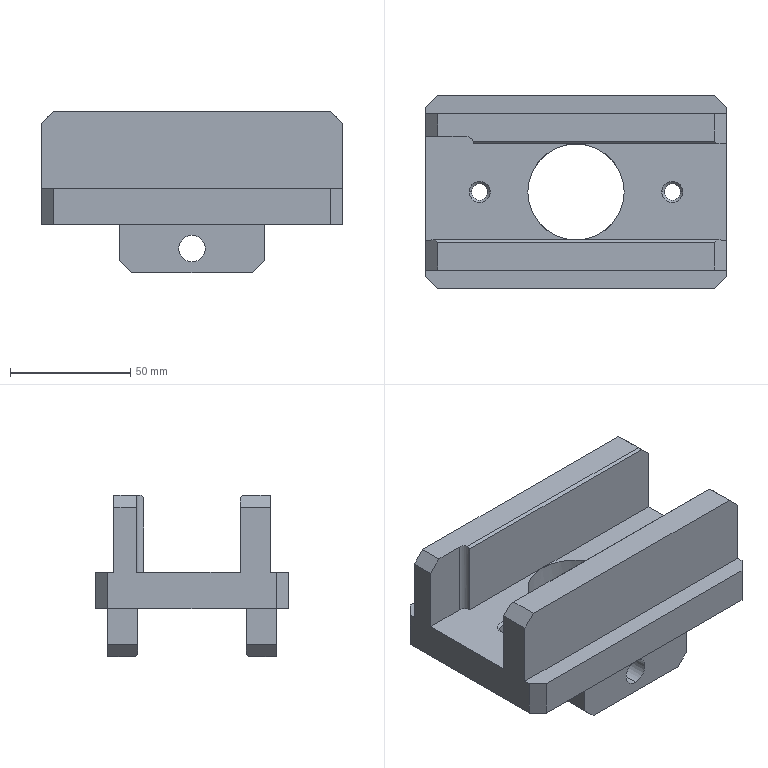Part | STEP file | YCD14007A-08.03.07.08 Gripper Seat | 1 solid | 59 faces | box 125 x 80 x 67 mm | volume 253618 mm3 | plane 42 | cylinder 11 | cone 6 | commonest cylinder face diameters 6.8 x4 11 x4 40 x2 6 x1